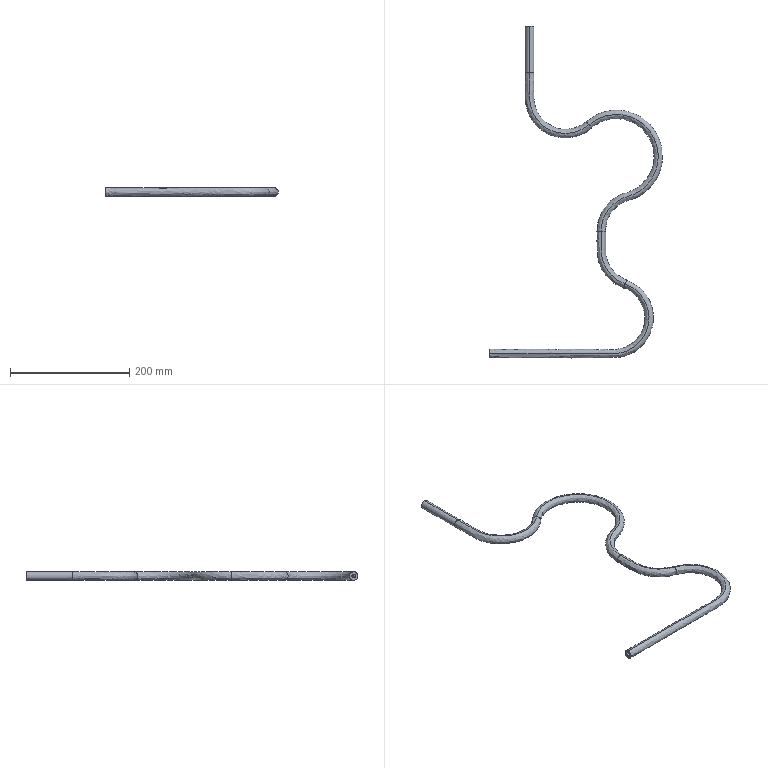Part | NX | features BREP 1 | 1 solid | 22 faces | box 289.489 x 555.807 x 14.509 mm | volume 140698 mm3 | spline 16 | cylinder 4 | plane 2 | commonest cylinder face diameters 6.35 x2 14.5 x2